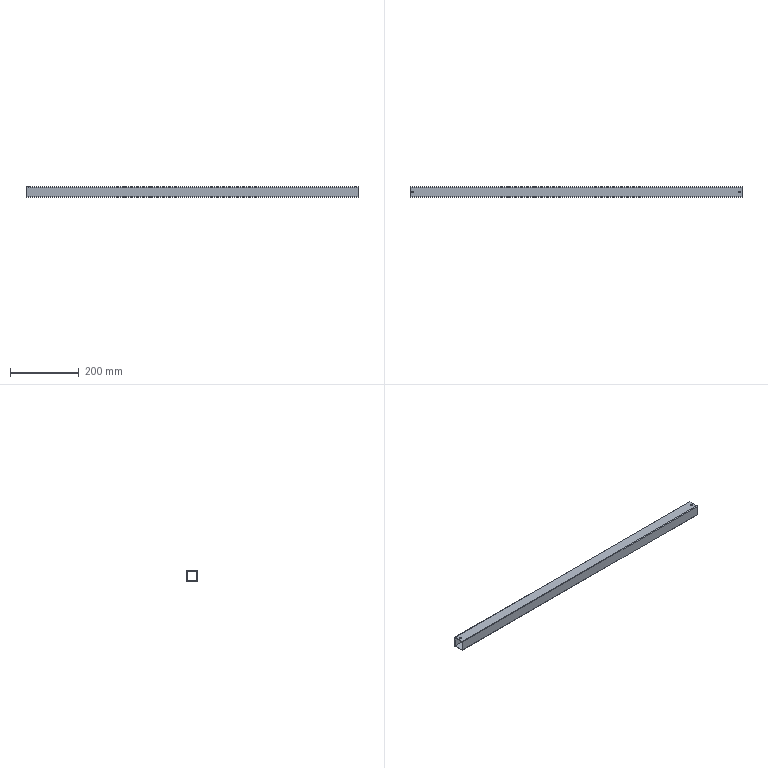Part | NX | features BREP 1 | 1 solid | 18 faces | box 965.2 x 31.75 x 31.75 mm | volume 214607 mm3 | plane 10 | cylinder 8 | commonest cylinder face diameters 3.175 x4 4.763 x4
STEP:
#1=CARTESIAN_POINT('',(-482.6,15.875,-14.287));
#2=VERTEX_POINT('',#1);
#3=CARTESIAN_POINT('',(-482.6,15.875,14.287));
#4=VERTEX_POINT('',#3);
#5=CARTESIAN_POINT('',(-482.6,15.875,-14.287));
#6=DIRECTION('',(0.,0.,1.));
#7=VECTOR('',#6,1000.);
#8=LINE('',#5,#7);
#9=EDGE_CURVE('',#2,#4,#8,.T.);
#10=ORIENTED_EDGE('',*,*,#9,.F.);
#11=CARTESIAN_POINT('',(-482.6,14.287,-15.875));
#12=VERTEX_POINT('',#11);
#13=CARTESIAN_POINT('',(-482.6,14.287,-14.287));
#14=DIRECTION('',(-1.,0.,0.));
#15=DIRECTION('',(0.,1.,0.));
#16=AXIS2_PLACEMENT_3D('',#13,#14,#15);
#17=CIRCLE('',#16,1.587);
#18=EDGE_CURVE('',#2,#12,#17,.T.);
#19=ORIENTED_EDGE('',*,*,#18,.T.);
#20=CARTESIAN_POINT('',(-482.6,-14.287,-15.875));
#21=VERTEX_POINT('',#20);
#22=CARTESIAN_POINT('',(-482.6,-14.287,-15.875));
#23=DIRECTION('',(0.,1.,0.));
#24=VECTOR('',#23,1000.);
#25=LINE('',#22,#24);
#26=EDGE_CURVE('',#21,#12,#25,.T.);
#27=ORIENTED_EDGE('',*,*,#26,.F.);
#28=CARTESIAN_POINT('',(-482.6,-15.875,-14.287));
#29=VERTEX_POINT('',#28);
#30=CARTESIAN_POINT('',(-482.6,-14.287,-14.287));
#31=DIRECTION('',(-1.,0.,0.));
#32=DIRECTION('',(0.,0.,-1.));
#33=AXIS2_PLACEMENT_3D('',#30,#31,#32);
#34=CIRCLE('',#33,1.587);
#35=EDGE_CURVE('',#21,#29,#34,.T.);
#36=ORIENTED_EDGE('',*,*,#35,.T.);
#37=CARTESIAN_POINT('',(-482.6,-15.875,14.287));
#38=VERTEX_POINT('',#37);
#39=CARTESIAN_POINT('',(-482.6,-15.875,14.287));
#40=DIRECTION('',(0.,0.,-1.));
#41=VECTOR('',#40,1000.);
#42=LINE('',#39,#41);
#43=EDGE_CURVE('',#38,#29,#42,.T.);
#44=ORIENTED_EDGE('',*,*,#43,.F.);
#45=CARTESIAN_POINT('',(-482.6,-14.287,15.875));
#46=VERTEX_POINT('',#45);
#47=CARTESIAN_POINT('',(-482.6,-14.287,14.287));
#48=DIRECTION('',(-1.,0.,0.));
#49=DIRECTION('',(0.,-1.,0.));
#50=AXIS2_PLACEMENT_3D('',#47,#48,#49);
#51=CIRCLE('',#50,1.587);
#52=EDGE_CURVE('',#38,#46,#51,.T.);
#53=ORIENTED_EDGE('',*,*,#52,.T.);
#54=CARTESIAN_POINT('',(-482.6,14.287,15.875));
#55=VERTEX_POINT('',#54);
#56=CARTESIAN_POINT('',(-482.6,14.287,15.875));
#57=DIRECTION('',(0.,-1.,0.));
#58=VECTOR('',#57,1000.);
#59=LINE('',#56,#58);
#60=EDGE_CURVE('',#55,#46,#59,.T.);
#61=ORIENTED_EDGE('',*,*,#60,.F.);
#62=CARTESIAN_POINT('',(-482.6,14.287,14.287));
#63=DIRECTION('',(-1.,0.,0.));
#64=DIRECTION('',(0.,0.,1.));
#65=AXIS2_PLACEMENT_3D('',#62,#63,#64);
#66=CIRCLE('',#65,1.587);
#67=EDGE_CURVE('',#55,#4,#66,.T.);
#68=ORIENTED_EDGE('',*,*,#67,.T.);
#69=EDGE_LOOP('',(#10,#19,#27,#36,#44,#53,#61,#68));
#70=FACE_BOUND('',#69,.T.);
#71=CARTESIAN_POINT('',(-482.6,13.995,13.995));
#72=VERTEX_POINT('',#71);
#73=CARTESIAN_POINT('',(-482.6,13.995,-13.995));
#74=VERTEX_POINT('',#73);
#75=CARTESIAN_POINT('',(-482.6,13.995,13.995));
#76=DIRECTION('',(0.,0.,-1.));
#77=VECTOR('',#76,1000.);
#78=LINE('',#75,#77);
#79=EDGE_CURVE('',#72,#74,#78,.T.);
#80=ORIENTED_EDGE('',*,*,#79,.F.);
#81=CARTESIAN_POINT('',(-482.6,-13.995,13.995));
#82=VERTEX_POINT('',#81);
#83=CARTESIAN_POINT('',(-482.6,-13.995,13.995));
#84=DIRECTION('',(0.,1.,0.));
#85=VECTOR('',#84,1000.);
#86=LINE('',#83,#85);
#87=EDGE_CURVE('',#82,#72,#86,.T.);
#88=ORIENTED_EDGE('',*,*,#87,.F.);
#89=CARTESIAN_POINT('',(-482.6,-13.995,-13.995));
#90=VERTEX_POINT('',#89);
#91=CARTESIAN_POINT('',(-482.6,-13.995,-13.995));
#92=DIRECTION('',(0.,0.,1.));
#93=VECTOR('',#92,1000.);
#94=LINE('',#91,#93);
#95=EDGE_CURVE('',#90,#82,#94,.T.);
#96=ORIENTED_EDGE('',*,*,#95,.F.);
#97=CARTESIAN_POINT('',(-482.6,13.995,-13.995));
#98=DIRECTION('',(0.,-1.,0.));
#99=VECTOR('',#98,1000.);
#100=LINE('',#97,#99);
#101=EDGE_CURVE('',#74,#90,#100,.T.);
#102=ORIENTED_EDGE('',*,*,#101,.F.);
#103=EDGE_LOOP('',(#80,#88,#96,#102));
#104=FACE_BOUND('',#103,.T.);
#105=CARTESIAN_POINT('',(-482.6,0.,0.));
#106=DIRECTION('',(1.,0.,0.));
#107=DIRECTION('',(0.,1.,0.));
#108=AXIS2_PLACEMENT_3D('',#105,#106,#107);
#109=PLANE('',#108);
#110=ADVANCED_FACE('',(#70,#104),#109,.F.);
#111=CARTESIAN_POINT('',(482.6,-13.995,-13.995));
#112=VERTEX_POINT('',#111);
#113=CARTESIAN_POINT('',(-482.6,-13.995,-13.995));
#114=DIRECTION('',(1.,0.,0.));
#115=VECTOR('',#114,1000.);
#116=LINE('',#113,#115);
#117=EDGE_CURVE('',#90,#112,#116,.T.);
#118=ORIENTED_EDGE('',*,*,#117,.T.);
#119=CARTESIAN_POINT('',(482.6,13.995,-13.995));
#120=VERTEX_POINT('',#119);
#121=CARTESIAN_POINT('',(482.6,13.995,-13.995));
#122=DIRECTION('',(0.,-1.,0.));
#123=VECTOR('',#122,1000.);
#124=LINE('',#121,#123);
#125=EDGE_CURVE('',#120,#112,#124,.T.);
#126=ORIENTED_EDGE('',*,*,#125,.F.);
#127=CARTESIAN_POINT('',(-482.6,13.995,-13.995));
#128=DIRECTION('',(1.,0.,0.));
#129=VECTOR('',#128,1000.);
#130=LINE('',#127,#129);
#131=EDGE_CURVE('',#74,#120,#130,.T.);
#132=ORIENTED_EDGE('',*,*,#131,.F.);
#133=ORIENTED_EDGE('',*,*,#101,.T.);
#134=EDGE_LOOP('',(#118,#126,#132,#133));
#135=FACE_BOUND('',#134,.T.);
#136=CARTESIAN_POINT('',(-482.6,13.995,-13.995));
#137=DIRECTION('',(0.,0.,1.));
#138=DIRECTION('',(1.,0.,0.));
#139=AXIS2_PLACEMENT_3D('',#136,#137,#138);
#140=PLANE('',#139);
#141=ADVANCED_FACE('',(#135),#140,.T.);
#142=ORIENTED_EDGE('',*,*,#131,.T.);
#143=CARTESIAN_POINT('',(482.6,13.995,13.995));
#144=VERTEX_POINT('',#143);
#145=CARTESIAN_POINT('',(482.6,13.995,13.995));
#146=DIRECTION('',(0.,0.,-1.));
#147=VECTOR('',#146,1000.);
#148=LINE('',#145,#147);
#149=EDGE_CURVE('',#144,#120,#148,.T.);
#150=ORIENTED_EDGE('',*,*,#149,.F.);
#151=CARTESIAN_POINT('',(-482.6,13.995,13.995));
#152=DIRECTION('',(1.,0.,0.));
#153=VECTOR('',#152,1000.);
#154=LINE('',#151,#153);
#155=EDGE_CURVE('',#72,#144,#154,.T.);
#156=ORIENTED_EDGE('',*,*,#155,.F.);
#157=ORIENTED_EDGE('',*,*,#79,.T.);
#158=EDGE_LOOP('',(#142,#150,#156,#157));
#159=FACE_BOUND('',#158,.T.);
#160=CARTESIAN_POINT('',(-482.6,13.995,13.995));
#161=DIRECTION('',(0.,-1.,0.));
#162=DIRECTION('',(0.,0.,-1.));
#163=AXIS2_PLACEMENT_3D('',#160,#161,#162);
#164=PLANE('',#163);
#165=ADVANCED_FACE('',(#159),#164,.T.);
#166=ORIENTED_EDGE('',*,*,#155,.T.);
#167=CARTESIAN_POINT('',(482.6,-13.995,13.995));
#168=VERTEX_POINT('',#167);
#169=CARTESIAN_POINT('',(482.6,-13.995,13.995));
#170=DIRECTION('',(0.,1.,0.));
#171=VECTOR('',#170,1000.);
#172=LINE('',#169,#171);
#173=EDGE_CURVE('',#168,#144,#172,.T.);
#174=ORIENTED_EDGE('',*,*,#173,.F.);
#175=CARTESIAN_POINT('',(-482.6,-13.995,13.995));
#176=DIRECTION('',(1.,0.,0.));
#177=VECTOR('',#176,1000.);
#178=LINE('',#175,#177);
#179=EDGE_CURVE('',#82,#168,#178,.T.);
#180=ORIENTED_EDGE('',*,*,#179,.F.);
#181=ORIENTED_EDGE('',*,*,#87,.T.);
#182=EDGE_LOOP('',(#166,#174,#180,#181));
#183=FACE_BOUND('',#182,.T.);
#184=CARTESIAN_POINT('',(476.98,0.,13.995));
#185=VERTEX_POINT('',#184);
#186=CARTESIAN_POINT('',(472.218,0.,13.995));
#187=VERTEX_POINT('',#186);
#188=CARTESIAN_POINT('',(474.599,0.,13.995));
#189=DIRECTION('',(0.,0.,-1.));
#190=DIRECTION('',(1.,0.,0.));
#191=AXIS2_PLACEMENT_3D('',#188,#189,#190);
#192=CIRCLE('',#191,2.381);
#193=EDGE_CURVE('',#185,#187,#192,.T.);
#194=ORIENTED_EDGE('',*,*,#193,.F.);
#195=CARTESIAN_POINT('',(474.599,0.,13.995));
#196=DIRECTION('',(0.,0.,-1.));
#197=DIRECTION('',(-1.,0.,0.));
#198=AXIS2_PLACEMENT_3D('',#195,#196,#197);
#199=CIRCLE('',#198,2.381);
#200=EDGE_CURVE('',#187,#185,#199,.T.);
#201=ORIENTED_EDGE('',*,*,#200,.F.);
#202=EDGE_LOOP('',(#194,#201));
#203=FACE_BOUND('',#202,.T.);
#204=CARTESIAN_POINT('',(-472.218,0.,13.995));
#205=VERTEX_POINT('',#204);
#206=CARTESIAN_POINT('',(-476.98,0.,13.995));
#207=VERTEX_POINT('',#206);
#208=CARTESIAN_POINT('',(-474.599,0.,13.995));
#209=DIRECTION('',(0.,0.,-1.));
#210=DIRECTION('',(1.,0.,0.));
#211=AXIS2_PLACEMENT_3D('',#208,#209,#210);
#212=CIRCLE('',#211,2.381);
#213=EDGE_CURVE('',#205,#207,#212,.T.);
#214=ORIENTED_EDGE('',*,*,#213,.F.);
#215=CARTESIAN_POINT('',(-474.599,0.,13.995));
#216=DIRECTION('',(0.,0.,-1.));
#217=DIRECTION('',(-1.,0.,0.));
#218=AXIS2_PLACEMENT_3D('',#215,#216,#217);
#219=CIRCLE('',#218,2.381);
#220=EDGE_CURVE('',#207,#205,#219,.T.);
#221=ORIENTED_EDGE('',*,*,#220,.F.);
#222=EDGE_LOOP('',(#214,#221));
#223=FACE_BOUND('',#222,.T.);
#224=CARTESIAN_POINT('',(-482.6,-13.995,13.995));
#225=DIRECTION('',(0.,0.,-1.));
#226=DIRECTION('',(0.,-1.,0.));
#227=AXIS2_PLACEMENT_3D('',#224,#225,#226);
#228=PLANE('',#227);
#229=ADVANCED_FACE('',(#183,#203,#223),#228,.T.);
#230=ORIENTED_EDGE('',*,*,#179,.T.);
#231=CARTESIAN_POINT('',(482.6,-13.995,-13.995));
#232=DIRECTION('',(0.,0.,1.));
#233=VECTOR('',#232,1000.);
#234=LINE('',#231,#233);
#235=EDGE_CURVE('',#112,#168,#234,.T.);
#236=ORIENTED_EDGE('',*,*,#235,.F.);
#237=ORIENTED_EDGE('',*,*,#117,.F.);
#238=ORIENTED_EDGE('',*,*,#95,.T.);
#239=EDGE_LOOP('',(#230,#236,#237,#238));
#240=FACE_BOUND('',#239,.T.);
#241=CARTESIAN_POINT('',(-482.6,-13.995,-13.995));
#242=DIRECTION('',(0.,1.,0.));
#243=DIRECTION('',(1.,0.,0.));
#244=AXIS2_PLACEMENT_3D('',#241,#242,#243);
#245=PLANE('',#244);
#246=ADVANCED_FACE('',(#240),#245,.T.);
#247=CARTESIAN_POINT('',(482.6,14.287,15.875));
#248=VERTEX_POINT('',#247);
#249=CARTESIAN_POINT('',(482.6,-14.287,15.875));
#250=VERTEX_POINT('',#249);
#251=CARTESIAN_POINT('',(482.6,14.287,15.875));
#252=DIRECTION('',(0.,-1.,0.));
#253=VECTOR('',#252,1000.);
#254=LINE('',#251,#253);
#255=EDGE_CURVE('',#248,#250,#254,.T.);
#256=ORIENTED_EDGE('',*,*,#255,.T.);
#257=CARTESIAN_POINT('',(482.6,-15.875,14.287));
#258=VERTEX_POINT('',#257);
#259=CARTESIAN_POINT('',(482.6,-14.287,14.287));
#260=DIRECTION('',(1.,0.,0.));
#261=DIRECTION('',(0.,0.,1.));
#262=AXIS2_PLACEMENT_3D('',#259,#260,#261);
#263=CIRCLE('',#262,1.587);
#264=EDGE_CURVE('',#250,#258,#263,.T.);
#265=ORIENTED_EDGE('',*,*,#264,.T.);
#266=CARTESIAN_POINT('',(482.6,-15.875,-14.287));
#267=VERTEX_POINT('',#266);
#268=CARTESIAN_POINT('',(482.6,-15.875,14.287));
#269=DIRECTION('',(0.,0.,-1.));
#270=VECTOR('',#269,1000.);
#271=LINE('',#268,#270);
#272=EDGE_CURVE('',#258,#267,#271,.T.);
#273=ORIENTED_EDGE('',*,*,#272,.T.);
#274=CARTESIAN_POINT('',(482.6,-14.287,-15.875));
#275=VERTEX_POINT('',#274);
#276=CARTESIAN_POINT('',(482.6,-14.287,-14.287));
#277=DIRECTION('',(1.,0.,0.));
#278=DIRECTION('',(0.,-1.,0.));
#279=AXIS2_PLACEMENT_3D('',#276,#277,#278);
#280=CIRCLE('',#279,1.587);
#281=EDGE_CURVE('',#267,#275,#280,.T.);
#282=ORIENTED_EDGE('',*,*,#281,.T.);
#283=CARTESIAN_POINT('',(482.6,14.287,-15.875));
#284=VERTEX_POINT('',#283);
#285=CARTESIAN_POINT('',(482.6,-14.287,-15.875));
#286=DIRECTION('',(0.,1.,0.));
#287=VECTOR('',#286,1000.);
#288=LINE('',#285,#287);
#289=EDGE_CURVE('',#275,#284,#288,.T.);
#290=ORIENTED_EDGE('',*,*,#289,.T.);
#291=CARTESIAN_POINT('',(482.6,15.875,-14.287));
#292=VERTEX_POINT('',#291);
#293=CARTESIAN_POINT('',(482.6,14.287,-14.287));
#294=DIRECTION('',(1.,0.,0.));
#295=DIRECTION('',(0.,0.,-1.));
#296=AXIS2_PLACEMENT_3D('',#293,#294,#295);
#297=CIRCLE('',#296,1.587);
#298=EDGE_CURVE('',#284,#292,#297,.T.);
#299=ORIENTED_EDGE('',*,*,#298,.T.);
#300=CARTESIAN_POINT('',(482.6,15.875,14.287));
#301=VERTEX_POINT('',#300);
#302=CARTESIAN_POINT('',(482.6,15.875,-14.287));
#303=DIRECTION('',(0.,0.,1.));
#304=VECTOR('',#303,1000.);
#305=LINE('',#302,#304);
#306=EDGE_CURVE('',#292,#301,#305,.T.);
#307=ORIENTED_EDGE('',*,*,#306,.T.);
#308=CARTESIAN_POINT('',(482.6,14.287,14.287));
#309=DIRECTION('',(1.,0.,0.));
#310=DIRECTION('',(0.,1.,0.));
#311=AXIS2_PLACEMENT_3D('',#308,#309,#310);
#312=CIRCLE('',#311,1.587);
#313=EDGE_CURVE('',#301,#248,#312,.T.);
#314=ORIENTED_EDGE('',*,*,#313,.T.);
#315=EDGE_LOOP('',(#256,#265,#273,#282,#290,#299,#307,#314));
#316=FACE_BOUND('',#315,.T.);
#317=ORIENTED_EDGE('',*,*,#235,.T.);
#318=ORIENTED_EDGE('',*,*,#173,.T.);
#319=ORIENTED_EDGE('',*,*,#149,.T.);
#320=ORIENTED_EDGE('',*,*,#125,.T.);
#321=EDGE_LOOP('',(#317,#318,#319,#320));
#322=FACE_BOUND('',#321,.T.);
#323=CARTESIAN_POINT('',(482.6,0.,0.));
#324=DIRECTION('',(1.,0.,0.));
#325=DIRECTION('',(0.,1.,0.));
#326=AXIS2_PLACEMENT_3D('',#323,#324,#325);
#327=PLANE('',#326);
#328=ADVANCED_FACE('',(#316,#322),#327,.T.);
#329=ORIENTED_EDGE('',*,*,#313,.F.);
#330=CARTESIAN_POINT('',(482.6,15.875,14.287));
#331=DIRECTION('',(-1.,0.,0.));
#332=VECTOR('',#331,1000.);
#333=LINE('',#330,#332);
#334=EDGE_CURVE('',#301,#4,#333,.T.);
#335=ORIENTED_EDGE('',*,*,#334,.T.);
#336=ORIENTED_EDGE('',*,*,#67,.F.);
#337=CARTESIAN_POINT('',(482.6,14.287,15.875));
#338=DIRECTION('',(-1.,0.,0.));
#339=VECTOR('',#338,1000.);
#340=LINE('',#337,#339);
#341=EDGE_CURVE('',#248,#55,#340,.T.);
#342=ORIENTED_EDGE('',*,*,#341,.F.);
#343=EDGE_LOOP('',(#329,#335,#336,#342));
#344=FACE_BOUND('',#343,.T.);
#345=CARTESIAN_POINT('',(484.112,14.287,14.287));
#346=DIRECTION('',(-1.,0.,0.));
#347=DIRECTION('',(0.,0.,1.));
#348=AXIS2_PLACEMENT_3D('',#345,#346,#347);
#349=CYLINDRICAL_SURFACE('',#348,1.587);
#350=ADVANCED_FACE('',(#344),#349,.T.);
#351=ORIENTED_EDGE('',*,*,#60,.T.);
#352=CARTESIAN_POINT('',(482.6,-14.287,15.875));
#353=DIRECTION('',(-1.,0.,0.));
#354=VECTOR('',#353,1000.);
#355=LINE('',#352,#354);
#356=EDGE_CURVE('',#250,#46,#355,.T.);
#357=ORIENTED_EDGE('',*,*,#356,.F.);
#358=ORIENTED_EDGE('',*,*,#255,.F.);
#359=ORIENTED_EDGE('',*,*,#341,.T.);
#360=EDGE_LOOP('',(#351,#357,#358,#359));
#361=FACE_BOUND('',#360,.T.);
#362=CARTESIAN_POINT('',(476.98,0.,15.875));
#363=VERTEX_POINT('',#362);
#364=CARTESIAN_POINT('',(472.218,0.,15.875));
#365=VERTEX_POINT('',#364);
#366=CARTESIAN_POINT('',(474.599,0.,15.875));
#367=DIRECTION('',(0.,0.,-1.));
#368=DIRECTION('',(1.,0.,0.));
#369=AXIS2_PLACEMENT_3D('',#366,#367,#368);
#370=CIRCLE('',#369,2.381);
#371=EDGE_CURVE('',#363,#365,#370,.T.);
#372=ORIENTED_EDGE('',*,*,#371,.T.);
#373=CARTESIAN_POINT('',(474.599,0.,15.875));
#374=DIRECTION('',(0.,0.,-1.));
#375=DIRECTION('',(-1.,0.,0.));
#376=AXIS2_PLACEMENT_3D('',#373,#374,#375);
#377=CIRCLE('',#376,2.381);
#378=EDGE_CURVE('',#365,#363,#377,.T.);
#379=ORIENTED_EDGE('',*,*,#378,.T.);
#380=EDGE_LOOP('',(#372,#379));
#381=FACE_BOUND('',#380,.T.);
#382=CARTESIAN_POINT('',(-472.218,0.,15.875));
#383=VERTEX_POINT('',#382);
#384=CARTESIAN_POINT('',(-476.98,0.,15.875));
#385=VERTEX_POINT('',#384);
#386=CARTESIAN_POINT('',(-474.599,0.,15.875));
#387=DIRECTION('',(0.,0.,-1.));
#388=DIRECTION('',(1.,0.,0.));
#389=AXIS2_PLACEMENT_3D('',#386,#387,#388);
#390=CIRCLE('',#389,2.381);
#391=EDGE_CURVE('',#383,#385,#390,.T.);
#392=ORIENTED_EDGE('',*,*,#391,.T.);
#393=CARTESIAN_POINT('',(-474.599,0.,15.875));
#394=DIRECTION('',(0.,0.,-1.));
#395=DIRECTION('',(-1.,0.,0.));
#396=AXIS2_PLACEMENT_3D('',#393,#394,#395);
#397=CIRCLE('',#396,2.381);
#398=EDGE_CURVE('',#385,#383,#397,.T.);
#399=ORIENTED_EDGE('',*,*,#398,.T.);
#400=EDGE_LOOP('',(#392,#399));
#401=FACE_BOUND('',#400,.T.);
#402=CARTESIAN_POINT('',(-482.6,15.875,15.875));
#403=DIRECTION('',(0.,0.,1.));
#404=DIRECTION('',(1.,0.,0.));
#405=AXIS2_PLACEMENT_3D('',#402,#403,#404);
#406=PLANE('',#405);
#407=ADVANCED_FACE('',(#361,#381,#401),#406,.T.);
#408=ORIENTED_EDGE('',*,*,#264,.F.);
#409=ORIENTED_EDGE('',*,*,#356,.T.);
#410=ORIENTED_EDGE('',*,*,#52,.F.);
#411=CARTESIAN_POINT('',(482.6,-15.875,14.287));
#412=DIRECTION('',(-1.,0.,0.));
#413=VECTOR('',#412,1000.);
#414=LINE('',#411,#413);
#415=EDGE_CURVE('',#258,#38,#414,.T.);
#416=ORIENTED_EDGE('',*,*,#415,.F.);
#417=EDGE_LOOP('',(#408,#409,#410,#416));
#418=FACE_BOUND('',#417,.T.);
#419=CARTESIAN_POINT('',(484.112,-14.287,14.287));
#420=DIRECTION('',(-1.,0.,0.));
#421=DIRECTION('',(0.,-1.,0.));
#422=AXIS2_PLACEMENT_3D('',#419,#420,#421);
#423=CYLINDRICAL_SURFACE('',#422,1.587);
#424=ADVANCED_FACE('',(#418),#423,.T.);
#425=ORIENTED_EDGE('',*,*,#43,.T.);
#426=CARTESIAN_POINT('',(482.6,-15.875,-14.287));
#427=DIRECTION('',(-1.,0.,0.));
#428=VECTOR('',#427,1000.);
#429=LINE('',#426,#428);
#430=EDGE_CURVE('',#267,#29,#429,.T.);
#431=ORIENTED_EDGE('',*,*,#430,.F.);
#432=ORIENTED_EDGE('',*,*,#272,.F.);
#433=ORIENTED_EDGE('',*,*,#415,.T.);
#434=EDGE_LOOP('',(#425,#431,#432,#433));
#435=FACE_BOUND('',#434,.T.);
#436=CARTESIAN_POINT('',(-482.6,-15.875,15.875));
#437=DIRECTION('',(0.,-1.,0.));
#438=DIRECTION('',(0.,0.,-1.));
#439=AXIS2_PLACEMENT_3D('',#436,#437,#438);
#440=PLANE('',#439);
#441=ADVANCED_FACE('',(#435),#440,.T.);
#442=ORIENTED_EDGE('',*,*,#281,.F.);
#443=ORIENTED_EDGE('',*,*,#430,.T.);
#444=ORIENTED_EDGE('',*,*,#35,.F.);
#445=CARTESIAN_POINT('',(482.6,-14.287,-15.875));
#446=DIRECTION('',(-1.,0.,0.));
#447=VECTOR('',#446,1000.);
#448=LINE('',#445,#447);
#449=EDGE_CURVE('',#275,#21,#448,.T.);
#450=ORIENTED_EDGE('',*,*,#449,.F.);
#451=EDGE_LOOP('',(#442,#443,#444,#450));
#452=FACE_BOUND('',#451,.T.);
#453=CARTESIAN_POINT('',(484.112,-14.287,-14.287));
#454=DIRECTION('',(-1.,0.,0.));
#455=DIRECTION('',(0.,0.,-1.));
#456=AXIS2_PLACEMENT_3D('',#453,#454,#455);
#457=CYLINDRICAL_SURFACE('',#456,1.587);
#458=ADVANCED_FACE('',(#452),#457,.T.);
#459=ORIENTED_EDGE('',*,*,#289,.F.);
#460=ORIENTED_EDGE('',*,*,#449,.T.);
#461=ORIENTED_EDGE('',*,*,#26,.T.);
#462=CARTESIAN_POINT('',(482.6,14.287,-15.875));
#463=DIRECTION('',(-1.,0.,0.));
#464=VECTOR('',#463,1000.);
#465=LINE('',#462,#464);
#466=EDGE_CURVE('',#284,#12,#465,.T.);
#467=ORIENTED_EDGE('',*,*,#466,.F.);
#468=EDGE_LOOP('',(#459,#460,#461,#467));
#469=FACE_BOUND('',#468,.T.);
#470=CARTESIAN_POINT('',(-482.6,-15.875,-15.875));
#471=DIRECTION('',(0.,0.,-1.));
#472=DIRECTION('',(0.,-1.,0.));
#473=AXIS2_PLACEMENT_3D('',#470,#471,#472);
#474=PLANE('',#473);
#475=ADVANCED_FACE('',(#469),#474,.T.);
#476=ORIENTED_EDGE('',*,*,#298,.F.);
#477=ORIENTED_EDGE('',*,*,#466,.T.);
#478=ORIENTED_EDGE('',*,*,#18,.F.);
#479=CARTESIAN_POINT('',(482.6,15.875,-14.287));
#480=DIRECTION('',(-1.,0.,0.));
#481=VECTOR('',#480,1000.);
#482=LINE('',#479,#481);
#483=EDGE_CURVE('',#292,#2,#482,.T.);
#484=ORIENTED_EDGE('',*,*,#483,.F.);
#485=EDGE_LOOP('',(#476,#477,#478,#484));
#486=FACE_BOUND('',#485,.T.);
#487=CARTESIAN_POINT('',(484.112,14.287,-14.287));
#488=DIRECTION('',(-1.,0.,0.));
#489=DIRECTION('',(0.,1.,0.));
#490=AXIS2_PLACEMENT_3D('',#487,#488,#489);
#491=CYLINDRICAL_SURFACE('',#490,1.587);
#492=ADVANCED_FACE('',(#486),#491,.T.);
#493=ORIENTED_EDGE('',*,*,#306,.F.);
#494=ORIENTED_EDGE('',*,*,#483,.T.);
#495=ORIENTED_EDGE('',*,*,#9,.T.);
#496=ORIENTED_EDGE('',*,*,#334,.F.);
#497=EDGE_LOOP('',(#493,#494,#495,#496));
#498=FACE_BOUND('',#497,.T.);
#499=CARTESIAN_POINT('',(-482.6,15.875,-15.875));
#500=DIRECTION('',(0.,1.,0.));
#501=DIRECTION('',(1.,0.,0.));
#502=AXIS2_PLACEMENT_3D('',#499,#500,#501);
#503=PLANE('',#502);
#504=ADVANCED_FACE('',(#498),#503,.T.);
#505=CARTESIAN_POINT('',(472.218,0.,15.875));
#506=DIRECTION('',(0.,0.,-1.));
#507=VECTOR('',#506,1000.);
#508=LINE('',#505,#507);
#509=EDGE_CURVE('',#365,#187,#508,.T.);
#510=ORIENTED_EDGE('',*,*,#509,.T.);
#511=ORIENTED_EDGE('',*,*,#200,.T.);
#512=CARTESIAN_POINT('',(476.98,0.,15.875));
#513=DIRECTION('',(0.,0.,-1.));
#514=VECTOR('',#513,1000.);
#515=LINE('',#512,#514);
#516=EDGE_CURVE('',#363,#185,#515,.T.);
#517=ORIENTED_EDGE('',*,*,#516,.F.);
#518=ORIENTED_EDGE('',*,*,#378,.F.);
#519=EDGE_LOOP('',(#510,#511,#517,#518));
#520=FACE_BOUND('',#519,.T.);
#521=CARTESIAN_POINT('',(474.599,0.,15.875));
#522=DIRECTION('',(0.,0.,-1.));
#523=DIRECTION('',(-1.,0.,0.));
#524=AXIS2_PLACEMENT_3D('',#521,#522,#523);
#525=CYLINDRICAL_SURFACE('',#524,2.381);
#526=ADVANCED_FACE('',(#520),#525,.F.);
#527=ORIENTED_EDGE('',*,*,#516,.T.);
#528=ORIENTED_EDGE('',*,*,#193,.T.);
#529=ORIENTED_EDGE('',*,*,#509,.F.);
#530=ORIENTED_EDGE('',*,*,#371,.F.);
#531=EDGE_LOOP('',(#527,#528,#529,#530));
#532=FACE_BOUND('',#531,.T.);
#533=CARTESIAN_POINT('',(474.599,0.,15.875));
#534=DIRECTION('',(0.,0.,-1.));
#535=DIRECTION('',(-1.,0.,0.));
#536=AXIS2_PLACEMENT_3D('',#533,#534,#535);
#537=CYLINDRICAL_SURFACE('',#536,2.381);
#538=ADVANCED_FACE('',(#532),#537,.F.);
#539=CARTESIAN_POINT('',(-476.98,0.,15.875));
#540=DIRECTION('',(0.,0.,-1.));
#541=VECTOR('',#540,1000.);
#542=LINE('',#539,#541);
#543=EDGE_CURVE('',#385,#207,#542,.T.);
#544=ORIENTED_EDGE('',*,*,#543,.T.);
#545=ORIENTED_EDGE('',*,*,#220,.T.);
#546=CARTESIAN_POINT('',(-472.218,0.,15.875));
#547=DIRECTION('',(0.,0.,-1.));
#548=VECTOR('',#547,1000.);
#549=LINE('',#546,#548);
#550=EDGE_CURVE('',#383,#205,#549,.T.);
#551=ORIENTED_EDGE('',*,*,#550,.F.);
#552=ORIENTED_EDGE('',*,*,#398,.F.);
#553=EDGE_LOOP('',(#544,#545,#551,#552));
#554=FACE_BOUND('',#553,.T.);
#555=CARTESIAN_POINT('',(-474.599,0.,15.875));
#556=DIRECTION('',(0.,0.,-1.));
#557=DIRECTION('',(-1.,0.,0.));
#558=AXIS2_PLACEMENT_3D('',#555,#556,#557);
#559=CYLINDRICAL_SURFACE('',#558,2.381);
#560=ADVANCED_FACE('',(#554),#559,.F.);
#561=ORIENTED_EDGE('',*,*,#550,.T.);
#562=ORIENTED_EDGE('',*,*,#213,.T.);
#563=ORIENTED_EDGE('',*,*,#543,.F.);
#564=ORIENTED_EDGE('',*,*,#391,.F.);
#565=EDGE_LOOP('',(#561,#562,#563,#564));
#566=FACE_BOUND('',#565,.T.);
#567=CARTESIAN_POINT('',(-474.599,0.,15.875));
#568=DIRECTION('',(0.,0.,-1.));
#569=DIRECTION('',(-1.,0.,0.));
#570=AXIS2_PLACEMENT_3D('',#567,#568,#569);
#571=CYLINDRICAL_SURFACE('',#570,2.381);
#572=ADVANCED_FACE('',(#566),#571,.F.);
#573=CLOSED_SHELL('',(#110,#141,#165,#229,#246,#328,#350,#407,#424,#441,#458,#475,#492,#504,#526,#538,#560,#572));
#574=MANIFOLD_SOLID_BREP('',#573);
#575=(LENGTH_UNIT()NAMED_UNIT(*)SI_UNIT(.MILLI.,.METRE.));
#576=UNCERTAINTY_MEASURE_WITH_UNIT(LENGTH_MEASURE(0.00001),#575,'','');
#577=(NAMED_UNIT(*)PLANE_ANGLE_UNIT()SI_UNIT($,.RADIAN.));
#578=(NAMED_UNIT(*)SI_UNIT($,.STERADIAN.)SOLID_ANGLE_UNIT());
#579=(GEOMETRIC_REPRESENTATION_CONTEXT(3)GLOBAL_UNCERTAINTY_ASSIGNED_CONTEXT((#576))GLOBAL_UNIT_ASSIGNED_CONTEXT((#575,#577,#578))REPRESENTATION_CONTEXT('',''));
#580=ADVANCED_BREP_SHAPE_REPRESENTATION('',(#574),#579);